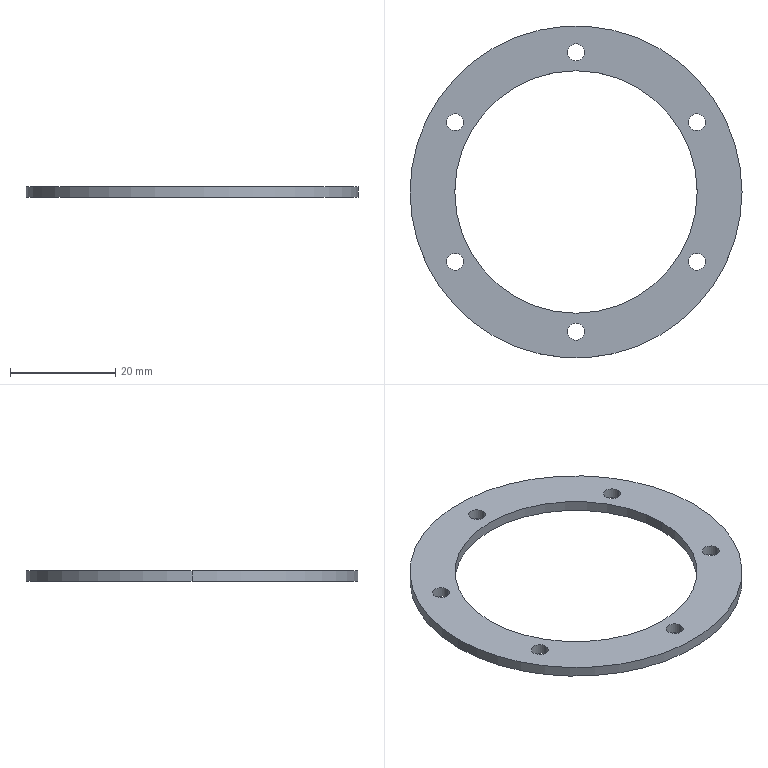Part | SolidWorks | features BaseBody 1 | 1 solid | 18 faces | box 63 x 63 x 2 mm | volume 2814 mm3 | cylinder 16 | plane 2 | commonest cylinder face diameters 3.2 x12 46 x2 63 x2
STEP:
#1=CARTESIAN_POINT('',(-21.35,13.25,2.));
#2=VERTEX_POINT('',#1);
#3=CARTESIAN_POINT('',(-24.55,13.25,2.));
#4=VERTEX_POINT('',#3);
#5=CARTESIAN_POINT('',(-22.95,13.25,2.));
#6=DIRECTION('',(0.,0.,-1.));
#7=DIRECTION('',(-1.,0.,0.));
#8=AXIS2_PLACEMENT_3D('',#5,#6,#7);
#9=CIRCLE('',#8,1.6);
#10=EDGE_CURVE('',#2,#4,#9,.T.);
#11=ORIENTED_EDGE('',*,*,#10,.F.);
#12=CARTESIAN_POINT('',(-21.35,13.25,0.));
#13=VERTEX_POINT('',#12);
#14=CARTESIAN_POINT('',(-21.35,13.25,2.));
#15=DIRECTION('',(0.,0.,-1.));
#16=VECTOR('',#15,1000.);
#17=LINE('',#14,#16);
#18=EDGE_CURVE('',#2,#13,#17,.T.);
#19=ORIENTED_EDGE('',*,*,#18,.T.);
#20=CARTESIAN_POINT('',(-24.55,13.25,0.));
#21=VERTEX_POINT('',#20);
#22=CARTESIAN_POINT('',(-22.95,13.25,0.));
#23=DIRECTION('',(0.,0.,1.));
#24=DIRECTION('',(-1.,0.,0.));
#25=AXIS2_PLACEMENT_3D('',#22,#23,#24);
#26=CIRCLE('',#25,1.6);
#27=EDGE_CURVE('',#21,#13,#26,.T.);
#28=ORIENTED_EDGE('',*,*,#27,.F.);
#29=CARTESIAN_POINT('',(-24.55,13.25,2.));
#30=DIRECTION('',(0.,0.,-1.));
#31=VECTOR('',#30,1000.);
#32=LINE('',#29,#31);
#33=EDGE_CURVE('',#4,#21,#32,.T.);
#34=ORIENTED_EDGE('',*,*,#33,.F.);
#35=EDGE_LOOP('',(#11,#19,#28,#34));
#36=FACE_OUTER_BOUND('',#35,.T.);
#37=CARTESIAN_POINT('',(-22.95,13.25,2.));
#38=DIRECTION('',(0.,0.,-1.));
#39=DIRECTION('',(-1.,0.,0.));
#40=AXIS2_PLACEMENT_3D('',#37,#38,#39);
#41=CYLINDRICAL_SURFACE('',#40,1.6);
#42=ADVANCED_FACE('',(#36),#41,.F.);
#43=CARTESIAN_POINT('',(1.6,-26.5,2.));
#44=VERTEX_POINT('',#43);
#45=CARTESIAN_POINT('',(-1.6,-26.5,2.));
#46=VERTEX_POINT('',#45);
#47=CARTESIAN_POINT('',(0.,-26.5,2.));
#48=DIRECTION('',(0.,0.,-1.));
#49=DIRECTION('',(-1.,0.,0.));
#50=AXIS2_PLACEMENT_3D('',#47,#48,#49);
#51=CIRCLE('',#50,1.6);
#52=EDGE_CURVE('',#44,#46,#51,.T.);
#53=ORIENTED_EDGE('',*,*,#52,.F.);
#54=CARTESIAN_POINT('',(1.6,-26.5,0.));
#55=VERTEX_POINT('',#54);
#56=CARTESIAN_POINT('',(1.6,-26.5,2.));
#57=DIRECTION('',(0.,0.,-1.));
#58=VECTOR('',#57,1000.);
#59=LINE('',#56,#58);
#60=EDGE_CURVE('',#44,#55,#59,.T.);
#61=ORIENTED_EDGE('',*,*,#60,.T.);
#62=CARTESIAN_POINT('',(-1.6,-26.5,0.));
#63=VERTEX_POINT('',#62);
#64=CARTESIAN_POINT('',(0.,-26.5,0.));
#65=DIRECTION('',(0.,0.,1.));
#66=DIRECTION('',(-1.,0.,0.));
#67=AXIS2_PLACEMENT_3D('',#64,#65,#66);
#68=CIRCLE('',#67,1.6);
#69=EDGE_CURVE('',#63,#55,#68,.T.);
#70=ORIENTED_EDGE('',*,*,#69,.F.);
#71=CARTESIAN_POINT('',(-1.6,-26.5,2.));
#72=DIRECTION('',(0.,0.,-1.));
#73=VECTOR('',#72,1000.);
#74=LINE('',#71,#73);
#75=EDGE_CURVE('',#46,#63,#74,.T.);
#76=ORIENTED_EDGE('',*,*,#75,.F.);
#77=EDGE_LOOP('',(#53,#61,#70,#76));
#78=FACE_OUTER_BOUND('',#77,.T.);
#79=CARTESIAN_POINT('',(0.,-26.5,2.));
#80=DIRECTION('',(0.,0.,-1.));
#81=DIRECTION('',(-1.,0.,0.));
#82=AXIS2_PLACEMENT_3D('',#79,#80,#81);
#83=CYLINDRICAL_SURFACE('',#82,1.6);
#84=ADVANCED_FACE('',(#78),#83,.F.);
#85=CARTESIAN_POINT('',(24.55,13.25,2.));
#86=VERTEX_POINT('',#85);
#87=CARTESIAN_POINT('',(21.35,13.25,2.));
#88=VERTEX_POINT('',#87);
#89=CARTESIAN_POINT('',(22.95,13.25,2.));
#90=DIRECTION('',(0.,0.,-1.));
#91=DIRECTION('',(-1.,0.,0.));
#92=AXIS2_PLACEMENT_3D('',#89,#90,#91);
#93=CIRCLE('',#92,1.6);
#94=EDGE_CURVE('',#86,#88,#93,.T.);
#95=ORIENTED_EDGE('',*,*,#94,.F.);
#96=CARTESIAN_POINT('',(24.55,13.25,0.));
#97=VERTEX_POINT('',#96);
#98=CARTESIAN_POINT('',(24.55,13.25,2.));
#99=DIRECTION('',(0.,0.,-1.));
#100=VECTOR('',#99,1000.);
#101=LINE('',#98,#100);
#102=EDGE_CURVE('',#86,#97,#101,.T.);
#103=ORIENTED_EDGE('',*,*,#102,.T.);
#104=CARTESIAN_POINT('',(21.35,13.25,0.));
#105=VERTEX_POINT('',#104);
#106=CARTESIAN_POINT('',(22.95,13.25,0.));
#107=DIRECTION('',(0.,0.,1.));
#108=DIRECTION('',(-1.,0.,0.));
#109=AXIS2_PLACEMENT_3D('',#106,#107,#108);
#110=CIRCLE('',#109,1.6);
#111=EDGE_CURVE('',#105,#97,#110,.T.);
#112=ORIENTED_EDGE('',*,*,#111,.F.);
#113=CARTESIAN_POINT('',(21.35,13.25,2.));
#114=DIRECTION('',(0.,0.,-1.));
#115=VECTOR('',#114,1000.);
#116=LINE('',#113,#115);
#117=EDGE_CURVE('',#88,#105,#116,.T.);
#118=ORIENTED_EDGE('',*,*,#117,.F.);
#119=EDGE_LOOP('',(#95,#103,#112,#118));
#120=FACE_OUTER_BOUND('',#119,.T.);
#121=CARTESIAN_POINT('',(22.95,13.25,2.));
#122=DIRECTION('',(0.,0.,-1.));
#123=DIRECTION('',(-1.,0.,0.));
#124=AXIS2_PLACEMENT_3D('',#121,#122,#123);
#125=CYLINDRICAL_SURFACE('',#124,1.6);
#126=ADVANCED_FACE('',(#120),#125,.F.);
#127=CARTESIAN_POINT('',(23.,0.,2.));
#128=VERTEX_POINT('',#127);
#129=CARTESIAN_POINT('',(-23.,0.,2.));
#130=VERTEX_POINT('',#129);
#131=CARTESIAN_POINT('',(0.,0.,2.));
#132=DIRECTION('',(0.,0.,-1.));
#133=DIRECTION('',(-1.,0.,0.));
#134=AXIS2_PLACEMENT_3D('',#131,#132,#133);
#135=CIRCLE('',#134,23.);
#136=EDGE_CURVE('',#128,#130,#135,.T.);
#137=ORIENTED_EDGE('',*,*,#136,.F.);
#138=CARTESIAN_POINT('',(23.,0.,0.));
#139=VERTEX_POINT('',#138);
#140=CARTESIAN_POINT('',(23.,0.,2.));
#141=DIRECTION('',(0.,0.,-1.));
#142=VECTOR('',#141,1000.);
#143=LINE('',#140,#142);
#144=EDGE_CURVE('',#128,#139,#143,.T.);
#145=ORIENTED_EDGE('',*,*,#144,.T.);
#146=CARTESIAN_POINT('',(-23.,0.,0.));
#147=VERTEX_POINT('',#146);
#148=CARTESIAN_POINT('',(0.,0.,0.));
#149=DIRECTION('',(0.,0.,1.));
#150=DIRECTION('',(-1.,0.,0.));
#151=AXIS2_PLACEMENT_3D('',#148,#149,#150);
#152=CIRCLE('',#151,23.);
#153=EDGE_CURVE('',#147,#139,#152,.T.);
#154=ORIENTED_EDGE('',*,*,#153,.F.);
#155=CARTESIAN_POINT('',(-23.,0.,2.));
#156=DIRECTION('',(0.,0.,-1.));
#157=VECTOR('',#156,1000.);
#158=LINE('',#155,#157);
#159=EDGE_CURVE('',#130,#147,#158,.T.);
#160=ORIENTED_EDGE('',*,*,#159,.F.);
#161=EDGE_LOOP('',(#137,#145,#154,#160));
#162=FACE_OUTER_BOUND('',#161,.T.);
#163=CARTESIAN_POINT('',(0.,0.,2.));
#164=DIRECTION('',(0.,0.,-1.));
#165=DIRECTION('',(-1.,0.,0.));
#166=AXIS2_PLACEMENT_3D('',#163,#164,#165);
#167=CYLINDRICAL_SURFACE('',#166,23.);
#168=ADVANCED_FACE('',(#162),#167,.F.);
#169=CARTESIAN_POINT('',(31.5,0.,2.));
#170=VERTEX_POINT('',#169);
#171=CARTESIAN_POINT('',(-31.5,0.,2.));
#172=VERTEX_POINT('',#171);
#173=CARTESIAN_POINT('',(0.,0.,2.));
#174=DIRECTION('',(0.,0.,1.));
#175=DIRECTION('',(-1.,0.,0.));
#176=AXIS2_PLACEMENT_3D('',#173,#174,#175);
#177=CIRCLE('',#176,31.5);
#178=EDGE_CURVE('',#170,#172,#177,.T.);
#179=ORIENTED_EDGE('',*,*,#178,.F.);
#180=CARTESIAN_POINT('',(31.5,0.,0.));
#181=VERTEX_POINT('',#180);
#182=CARTESIAN_POINT('',(31.5,0.,2.));
#183=DIRECTION('',(0.,0.,-1.));
#184=VECTOR('',#183,1000.);
#185=LINE('',#182,#184);
#186=EDGE_CURVE('',#170,#181,#185,.T.);
#187=ORIENTED_EDGE('',*,*,#186,.T.);
#188=CARTESIAN_POINT('',(-31.5,0.,0.));
#189=VERTEX_POINT('',#188);
#190=CARTESIAN_POINT('',(0.,0.,0.));
#191=DIRECTION('',(0.,0.,1.));
#192=DIRECTION('',(-1.,0.,0.));
#193=AXIS2_PLACEMENT_3D('',#190,#191,#192);
#194=CIRCLE('',#193,31.5);
#195=EDGE_CURVE('',#181,#189,#194,.T.);
#196=ORIENTED_EDGE('',*,*,#195,.T.);
#197=CARTESIAN_POINT('',(-31.5,0.,2.));
#198=DIRECTION('',(0.,0.,-1.));
#199=VECTOR('',#198,1000.);
#200=LINE('',#197,#199);
#201=EDGE_CURVE('',#172,#189,#200,.T.);
#202=ORIENTED_EDGE('',*,*,#201,.F.);
#203=EDGE_LOOP('',(#179,#187,#196,#202));
#204=FACE_OUTER_BOUND('',#203,.T.);
#205=CARTESIAN_POINT('',(0.,0.,2.));
#206=DIRECTION('',(0.,0.,-1.));
#207=DIRECTION('',(-1.,0.,0.));
#208=AXIS2_PLACEMENT_3D('',#205,#206,#207);
#209=CYLINDRICAL_SURFACE('',#208,31.5);
#210=ADVANCED_FACE('',(#204),#209,.T.);
#211=CARTESIAN_POINT('',(1.6,26.5,2.));
#212=VERTEX_POINT('',#211);
#213=CARTESIAN_POINT('',(-1.6,26.5,2.));
#214=VERTEX_POINT('',#213);
#215=CARTESIAN_POINT('',(0.,26.5,2.));
#216=DIRECTION('',(0.,0.,-1.));
#217=DIRECTION('',(-1.,0.,0.));
#218=AXIS2_PLACEMENT_3D('',#215,#216,#217);
#219=CIRCLE('',#218,1.6);
#220=EDGE_CURVE('',#212,#214,#219,.T.);
#221=ORIENTED_EDGE('',*,*,#220,.F.);
#222=CARTESIAN_POINT('',(1.6,26.5,0.));
#223=VERTEX_POINT('',#222);
#224=CARTESIAN_POINT('',(1.6,26.5,2.));
#225=DIRECTION('',(0.,0.,-1.));
#226=VECTOR('',#225,1000.);
#227=LINE('',#224,#226);
#228=EDGE_CURVE('',#212,#223,#227,.T.);
#229=ORIENTED_EDGE('',*,*,#228,.T.);
#230=CARTESIAN_POINT('',(-1.6,26.5,0.));
#231=VERTEX_POINT('',#230);
#232=CARTESIAN_POINT('',(0.,26.5,0.));
#233=DIRECTION('',(0.,0.,1.));
#234=DIRECTION('',(-1.,0.,0.));
#235=AXIS2_PLACEMENT_3D('',#232,#233,#234);
#236=CIRCLE('',#235,1.6);
#237=EDGE_CURVE('',#231,#223,#236,.T.);
#238=ORIENTED_EDGE('',*,*,#237,.F.);
#239=CARTESIAN_POINT('',(-1.6,26.5,2.));
#240=DIRECTION('',(0.,0.,-1.));
#241=VECTOR('',#240,1000.);
#242=LINE('',#239,#241);
#243=EDGE_CURVE('',#214,#231,#242,.T.);
#244=ORIENTED_EDGE('',*,*,#243,.F.);
#245=EDGE_LOOP('',(#221,#229,#238,#244));
#246=FACE_OUTER_BOUND('',#245,.T.);
#247=CARTESIAN_POINT('',(0.,26.5,2.));
#248=DIRECTION('',(0.,0.,-1.));
#249=DIRECTION('',(-1.,0.,0.));
#250=AXIS2_PLACEMENT_3D('',#247,#248,#249);
#251=CYLINDRICAL_SURFACE('',#250,1.6);
#252=ADVANCED_FACE('',(#246),#251,.F.);
#253=CARTESIAN_POINT('',(24.55,-13.25,2.));
#254=VERTEX_POINT('',#253);
#255=CARTESIAN_POINT('',(21.35,-13.25,2.));
#256=VERTEX_POINT('',#255);
#257=CARTESIAN_POINT('',(22.95,-13.25,2.));
#258=DIRECTION('',(0.,0.,-1.));
#259=DIRECTION('',(-1.,0.,0.));
#260=AXIS2_PLACEMENT_3D('',#257,#258,#259);
#261=CIRCLE('',#260,1.6);
#262=EDGE_CURVE('',#254,#256,#261,.T.);
#263=ORIENTED_EDGE('',*,*,#262,.F.);
#264=CARTESIAN_POINT('',(24.55,-13.25,0.));
#265=VERTEX_POINT('',#264);
#266=CARTESIAN_POINT('',(24.55,-13.25,2.));
#267=DIRECTION('',(0.,0.,-1.));
#268=VECTOR('',#267,1000.);
#269=LINE('',#266,#268);
#270=EDGE_CURVE('',#254,#265,#269,.T.);
#271=ORIENTED_EDGE('',*,*,#270,.T.);
#272=CARTESIAN_POINT('',(21.35,-13.25,0.));
#273=VERTEX_POINT('',#272);
#274=CARTESIAN_POINT('',(22.95,-13.25,0.));
#275=DIRECTION('',(0.,0.,1.));
#276=DIRECTION('',(-1.,0.,0.));
#277=AXIS2_PLACEMENT_3D('',#274,#275,#276);
#278=CIRCLE('',#277,1.6);
#279=EDGE_CURVE('',#273,#265,#278,.T.);
#280=ORIENTED_EDGE('',*,*,#279,.F.);
#281=CARTESIAN_POINT('',(21.35,-13.25,2.));
#282=DIRECTION('',(0.,0.,-1.));
#283=VECTOR('',#282,1000.);
#284=LINE('',#281,#283);
#285=EDGE_CURVE('',#256,#273,#284,.T.);
#286=ORIENTED_EDGE('',*,*,#285,.F.);
#287=EDGE_LOOP('',(#263,#271,#280,#286));
#288=FACE_OUTER_BOUND('',#287,.T.);
#289=CARTESIAN_POINT('',(22.95,-13.25,2.));
#290=DIRECTION('',(0.,0.,-1.));
#291=DIRECTION('',(-1.,0.,0.));
#292=AXIS2_PLACEMENT_3D('',#289,#290,#291);
#293=CYLINDRICAL_SURFACE('',#292,1.6);
#294=ADVANCED_FACE('',(#288),#293,.F.);
#295=CARTESIAN_POINT('',(-21.35,-13.25,2.));
#296=VERTEX_POINT('',#295);
#297=CARTESIAN_POINT('',(-24.55,-13.25,2.));
#298=VERTEX_POINT('',#297);
#299=CARTESIAN_POINT('',(-22.95,-13.25,2.));
#300=DIRECTION('',(0.,0.,-1.));
#301=DIRECTION('',(-1.,0.,0.));
#302=AXIS2_PLACEMENT_3D('',#299,#300,#301);
#303=CIRCLE('',#302,1.6);
#304=EDGE_CURVE('',#296,#298,#303,.T.);
#305=ORIENTED_EDGE('',*,*,#304,.F.);
#306=CARTESIAN_POINT('',(-21.35,-13.25,0.));
#307=VERTEX_POINT('',#306);
#308=CARTESIAN_POINT('',(-21.35,-13.25,2.));
#309=DIRECTION('',(0.,0.,-1.));
#310=VECTOR('',#309,1000.);
#311=LINE('',#308,#310);
#312=EDGE_CURVE('',#296,#307,#311,.T.);
#313=ORIENTED_EDGE('',*,*,#312,.T.);
#314=CARTESIAN_POINT('',(-24.55,-13.25,0.));
#315=VERTEX_POINT('',#314);
#316=CARTESIAN_POINT('',(-22.95,-13.25,0.));
#317=DIRECTION('',(0.,0.,1.));
#318=DIRECTION('',(-1.,0.,0.));
#319=AXIS2_PLACEMENT_3D('',#316,#317,#318);
#320=CIRCLE('',#319,1.6);
#321=EDGE_CURVE('',#315,#307,#320,.T.);
#322=ORIENTED_EDGE('',*,*,#321,.F.);
#323=CARTESIAN_POINT('',(-24.55,-13.25,2.));
#324=DIRECTION('',(0.,0.,-1.));
#325=VECTOR('',#324,1000.);
#326=LINE('',#323,#325);
#327=EDGE_CURVE('',#298,#315,#326,.T.);
#328=ORIENTED_EDGE('',*,*,#327,.F.);
#329=EDGE_LOOP('',(#305,#313,#322,#328));
#330=FACE_OUTER_BOUND('',#329,.T.);
#331=CARTESIAN_POINT('',(-22.95,-13.25,2.));
#332=DIRECTION('',(0.,0.,-1.));
#333=DIRECTION('',(-1.,0.,0.));
#334=AXIS2_PLACEMENT_3D('',#331,#332,#333);
#335=CYLINDRICAL_SURFACE('',#334,1.6);
#336=ADVANCED_FACE('',(#330),#335,.F.);
#337=CARTESIAN_POINT('',(-22.95,13.25,2.));
#338=DIRECTION('',(0.,0.,-1.));
#339=DIRECTION('',(-1.,0.,0.));
#340=AXIS2_PLACEMENT_3D('',#337,#338,#339);
#341=CIRCLE('',#340,1.6);
#342=EDGE_CURVE('',#4,#2,#341,.T.);
#343=ORIENTED_EDGE('',*,*,#342,.T.);
#344=ORIENTED_EDGE('',*,*,#10,.T.);
#345=EDGE_LOOP('',(#343,#344));
#346=FACE_BOUND('',#345,.T.);
#347=CARTESIAN_POINT('',(0.,-26.5,2.));
#348=DIRECTION('',(0.,0.,-1.));
#349=DIRECTION('',(-1.,0.,0.));
#350=AXIS2_PLACEMENT_3D('',#347,#348,#349);
#351=CIRCLE('',#350,1.6);
#352=EDGE_CURVE('',#46,#44,#351,.T.);
#353=ORIENTED_EDGE('',*,*,#352,.T.);
#354=ORIENTED_EDGE('',*,*,#52,.T.);
#355=EDGE_LOOP('',(#353,#354));
#356=FACE_BOUND('',#355,.T.);
#357=CARTESIAN_POINT('',(22.95,13.25,2.));
#358=DIRECTION('',(0.,0.,-1.));
#359=DIRECTION('',(-1.,0.,0.));
#360=AXIS2_PLACEMENT_3D('',#357,#358,#359);
#361=CIRCLE('',#360,1.6);
#362=EDGE_CURVE('',#88,#86,#361,.T.);
#363=ORIENTED_EDGE('',*,*,#362,.T.);
#364=ORIENTED_EDGE('',*,*,#94,.T.);
#365=EDGE_LOOP('',(#363,#364));
#366=FACE_BOUND('',#365,.T.);
#367=CARTESIAN_POINT('',(0.,0.,2.));
#368=DIRECTION('',(0.,0.,-1.));
#369=DIRECTION('',(-1.,0.,0.));
#370=AXIS2_PLACEMENT_3D('',#367,#368,#369);
#371=CIRCLE('',#370,23.);
#372=EDGE_CURVE('',#130,#128,#371,.T.);
#373=ORIENTED_EDGE('',*,*,#372,.T.);
#374=ORIENTED_EDGE('',*,*,#136,.T.);
#375=EDGE_LOOP('',(#373,#374));
#376=FACE_BOUND('',#375,.T.);
#377=CARTESIAN_POINT('',(0.,0.,2.));
#378=DIRECTION('',(0.,0.,1.));
#379=DIRECTION('',(-1.,0.,0.));
#380=AXIS2_PLACEMENT_3D('',#377,#378,#379);
#381=CIRCLE('',#380,31.5);
#382=EDGE_CURVE('',#172,#170,#381,.T.);
#383=ORIENTED_EDGE('',*,*,#382,.T.);
#384=ORIENTED_EDGE('',*,*,#178,.T.);
#385=EDGE_LOOP('',(#383,#384));
#386=FACE_OUTER_BOUND('',#385,.T.);
#387=CARTESIAN_POINT('',(0.,26.5,2.));
#388=DIRECTION('',(0.,0.,-1.));
#389=DIRECTION('',(-1.,0.,0.));
#390=AXIS2_PLACEMENT_3D('',#387,#388,#389);
#391=CIRCLE('',#390,1.6);
#392=EDGE_CURVE('',#214,#212,#391,.T.);
#393=ORIENTED_EDGE('',*,*,#392,.T.);
#394=ORIENTED_EDGE('',*,*,#220,.T.);
#395=EDGE_LOOP('',(#393,#394));
#396=FACE_BOUND('',#395,.T.);
#397=CARTESIAN_POINT('',(22.95,-13.25,2.));
#398=DIRECTION('',(0.,0.,-1.));
#399=DIRECTION('',(-1.,0.,0.));
#400=AXIS2_PLACEMENT_3D('',#397,#398,#399);
#401=CIRCLE('',#400,1.6);
#402=EDGE_CURVE('',#256,#254,#401,.T.);
#403=ORIENTED_EDGE('',*,*,#402,.T.);
#404=ORIENTED_EDGE('',*,*,#262,.T.);
#405=EDGE_LOOP('',(#403,#404));
#406=FACE_BOUND('',#405,.T.);
#407=CARTESIAN_POINT('',(-22.95,-13.25,2.));
#408=DIRECTION('',(0.,0.,-1.));
#409=DIRECTION('',(-1.,0.,0.));
#410=AXIS2_PLACEMENT_3D('',#407,#408,#409);
#411=CIRCLE('',#410,1.6);
#412=EDGE_CURVE('',#298,#296,#411,.T.);
#413=ORIENTED_EDGE('',*,*,#412,.T.);
#414=ORIENTED_EDGE('',*,*,#304,.T.);
#415=EDGE_LOOP('',(#413,#414));
#416=FACE_BOUND('',#415,.T.);
#417=CARTESIAN_POINT('',(0.,0.,2.));
#418=DIRECTION('',(0.,0.,1.));
#419=DIRECTION('',(1.,0.,0.));
#420=AXIS2_PLACEMENT_3D('',#417,#418,#419);
#421=PLANE('',#420);
#422=ADVANCED_FACE('',(#346,#356,#366,#376,#386,#396,#406,#416),#421,.T.);
#423=ORIENTED_EDGE('',*,*,#18,.F.);
#424=ORIENTED_EDGE('',*,*,#342,.F.);
#425=ORIENTED_EDGE('',*,*,#33,.T.);
#426=CARTESIAN_POINT('',(-22.95,13.25,0.));
#427=DIRECTION('',(0.,0.,1.));
#428=DIRECTION('',(-1.,0.,0.));
#429=AXIS2_PLACEMENT_3D('',#426,#427,#428);
#430=CIRCLE('',#429,1.6);
#431=EDGE_CURVE('',#13,#21,#430,.T.);
#432=ORIENTED_EDGE('',*,*,#431,.F.);
#433=EDGE_LOOP('',(#423,#424,#425,#432));
#434=FACE_OUTER_BOUND('',#433,.T.);
#435=CARTESIAN_POINT('',(-22.95,13.25,2.));
#436=DIRECTION('',(0.,0.,-1.));
#437=DIRECTION('',(-1.,0.,0.));
#438=AXIS2_PLACEMENT_3D('',#435,#436,#437);
#439=CYLINDRICAL_SURFACE('',#438,1.6);
#440=ADVANCED_FACE('',(#434),#439,.F.);
#441=ORIENTED_EDGE('',*,*,#60,.F.);
#442=ORIENTED_EDGE('',*,*,#352,.F.);
#443=ORIENTED_EDGE('',*,*,#75,.T.);
#444=CARTESIAN_POINT('',(0.,-26.5,0.));
#445=DIRECTION('',(0.,0.,1.));
#446=DIRECTION('',(-1.,0.,0.));
#447=AXIS2_PLACEMENT_3D('',#444,#445,#446);
#448=CIRCLE('',#447,1.6);
#449=EDGE_CURVE('',#55,#63,#448,.T.);
#450=ORIENTED_EDGE('',*,*,#449,.F.);
#451=EDGE_LOOP('',(#441,#442,#443,#450));
#452=FACE_OUTER_BOUND('',#451,.T.);
#453=CARTESIAN_POINT('',(0.,-26.5,2.));
#454=DIRECTION('',(0.,0.,-1.));
#455=DIRECTION('',(-1.,0.,0.));
#456=AXIS2_PLACEMENT_3D('',#453,#454,#455);
#457=CYLINDRICAL_SURFACE('',#456,1.6);
#458=ADVANCED_FACE('',(#452),#457,.F.);
#459=ORIENTED_EDGE('',*,*,#102,.F.);
#460=ORIENTED_EDGE('',*,*,#362,.F.);
#461=ORIENTED_EDGE('',*,*,#117,.T.);
#462=CARTESIAN_POINT('',(22.95,13.25,0.));
#463=DIRECTION('',(0.,0.,1.));
#464=DIRECTION('',(-1.,0.,0.));
#465=AXIS2_PLACEMENT_3D('',#462,#463,#464);
#466=CIRCLE('',#465,1.6);
#467=EDGE_CURVE('',#97,#105,#466,.T.);
#468=ORIENTED_EDGE('',*,*,#467,.F.);
#469=EDGE_LOOP('',(#459,#460,#461,#468));
#470=FACE_OUTER_BOUND('',#469,.T.);
#471=CARTESIAN_POINT('',(22.95,13.25,2.));
#472=DIRECTION('',(0.,0.,-1.));
#473=DIRECTION('',(-1.,0.,0.));
#474=AXIS2_PLACEMENT_3D('',#471,#472,#473);
#475=CYLINDRICAL_SURFACE('',#474,1.6);
#476=ADVANCED_FACE('',(#470),#475,.F.);
#477=ORIENTED_EDGE('',*,*,#144,.F.);
#478=ORIENTED_EDGE('',*,*,#372,.F.);
#479=ORIENTED_EDGE('',*,*,#159,.T.);
#480=CARTESIAN_POINT('',(0.,0.,0.));
#481=DIRECTION('',(0.,0.,1.));
#482=DIRECTION('',(-1.,0.,0.));
#483=AXIS2_PLACEMENT_3D('',#480,#481,#482);
#484=CIRCLE('',#483,23.);
#485=EDGE_CURVE('',#139,#147,#484,.T.);
#486=ORIENTED_EDGE('',*,*,#485,.F.);
#487=EDGE_LOOP('',(#477,#478,#479,#486));
#488=FACE_OUTER_BOUND('',#487,.T.);
#489=CARTESIAN_POINT('',(0.,0.,2.));
#490=DIRECTION('',(0.,0.,-1.));
#491=DIRECTION('',(-1.,0.,0.));
#492=AXIS2_PLACEMENT_3D('',#489,#490,#491);
#493=CYLINDRICAL_SURFACE('',#492,23.);
#494=ADVANCED_FACE('',(#488),#493,.F.);
#495=ORIENTED_EDGE('',*,*,#186,.F.);
#496=ORIENTED_EDGE('',*,*,#382,.F.);
#497=ORIENTED_EDGE('',*,*,#201,.T.);
#498=CARTESIAN_POINT('',(0.,0.,0.));
#499=DIRECTION('',(0.,0.,1.));
#500=DIRECTION('',(-1.,0.,0.));
#501=AXIS2_PLACEMENT_3D('',#498,#499,#500);
#502=CIRCLE('',#501,31.5);
#503=EDGE_CURVE('',#189,#181,#502,.T.);
#504=ORIENTED_EDGE('',*,*,#503,.T.);
#505=EDGE_LOOP('',(#495,#496,#497,#504));
#506=FACE_OUTER_BOUND('',#505,.T.);
#507=CARTESIAN_POINT('',(0.,0.,2.));
#508=DIRECTION('',(0.,0.,-1.));
#509=DIRECTION('',(-1.,0.,0.));
#510=AXIS2_PLACEMENT_3D('',#507,#508,#509);
#511=CYLINDRICAL_SURFACE('',#510,31.5);
#512=ADVANCED_FACE('',(#506),#511,.T.);
#513=ORIENTED_EDGE('',*,*,#228,.F.);
#514=ORIENTED_EDGE('',*,*,#392,.F.);
#515=ORIENTED_EDGE('',*,*,#243,.T.);
#516=CARTESIAN_POINT('',(0.,26.5,0.));
#517=DIRECTION('',(0.,0.,1.));
#518=DIRECTION('',(-1.,0.,0.));
#519=AXIS2_PLACEMENT_3D('',#516,#517,#518);
#520=CIRCLE('',#519,1.6);
#521=EDGE_CURVE('',#223,#231,#520,.T.);
#522=ORIENTED_EDGE('',*,*,#521,.F.);
#523=EDGE_LOOP('',(#513,#514,#515,#522));
#524=FACE_OUTER_BOUND('',#523,.T.);
#525=CARTESIAN_POINT('',(0.,26.5,2.));
#526=DIRECTION('',(0.,0.,-1.));
#527=DIRECTION('',(-1.,0.,0.));
#528=AXIS2_PLACEMENT_3D('',#525,#526,#527);
#529=CYLINDRICAL_SURFACE('',#528,1.6);
#530=ADVANCED_FACE('',(#524),#529,.F.);
#531=ORIENTED_EDGE('',*,*,#270,.F.);
#532=ORIENTED_EDGE('',*,*,#402,.F.);
#533=ORIENTED_EDGE('',*,*,#285,.T.);
#534=CARTESIAN_POINT('',(22.95,-13.25,0.));
#535=DIRECTION('',(0.,0.,1.));
#536=DIRECTION('',(-1.,0.,0.));
#537=AXIS2_PLACEMENT_3D('',#534,#535,#536);
#538=CIRCLE('',#537,1.6);
#539=EDGE_CURVE('',#265,#273,#538,.T.);
#540=ORIENTED_EDGE('',*,*,#539,.F.);
#541=EDGE_LOOP('',(#531,#532,#533,#540));
#542=FACE_OUTER_BOUND('',#541,.T.);
#543=CARTESIAN_POINT('',(22.95,-13.25,2.));
#544=DIRECTION('',(0.,0.,-1.));
#545=DIRECTION('',(-1.,0.,0.));
#546=AXIS2_PLACEMENT_3D('',#543,#544,#545);
#547=CYLINDRICAL_SURFACE('',#546,1.6);
#548=ADVANCED_FACE('',(#542),#547,.F.);
#549=ORIENTED_EDGE('',*,*,#312,.F.);
#550=ORIENTED_EDGE('',*,*,#412,.F.);
#551=ORIENTED_EDGE('',*,*,#327,.T.);
#552=CARTESIAN_POINT('',(-22.95,-13.25,0.));
#553=DIRECTION('',(0.,0.,1.));
#554=DIRECTION('',(-1.,0.,0.));
#555=AXIS2_PLACEMENT_3D('',#552,#553,#554);
#556=CIRCLE('',#555,1.6);
#557=EDGE_CURVE('',#307,#315,#556,.T.);
#558=ORIENTED_EDGE('',*,*,#557,.F.);
#559=EDGE_LOOP('',(#549,#550,#551,#558));
#560=FACE_OUTER_BOUND('',#559,.T.);
#561=CARTESIAN_POINT('',(-22.95,-13.25,2.));
#562=DIRECTION('',(0.,0.,-1.));
#563=DIRECTION('',(-1.,0.,0.));
#564=AXIS2_PLACEMENT_3D('',#561,#562,#563);
#565=CYLINDRICAL_SURFACE('',#564,1.6);
#566=ADVANCED_FACE('',(#560),#565,.F.);
#567=ORIENTED_EDGE('',*,*,#27,.T.);
#568=ORIENTED_EDGE('',*,*,#431,.T.);
#569=EDGE_LOOP('',(#567,#568));
#570=FACE_BOUND('',#569,.T.);
#571=ORIENTED_EDGE('',*,*,#321,.T.);
#572=ORIENTED_EDGE('',*,*,#557,.T.);
#573=EDGE_LOOP('',(#571,#572));
#574=FACE_BOUND('',#573,.T.);
#575=ORIENTED_EDGE('',*,*,#69,.T.);
#576=ORIENTED_EDGE('',*,*,#449,.T.);
#577=EDGE_LOOP('',(#575,#576));
#578=FACE_BOUND('',#577,.T.);
#579=ORIENTED_EDGE('',*,*,#279,.T.);
#580=ORIENTED_EDGE('',*,*,#539,.T.);
#581=EDGE_LOOP('',(#579,#580));
#582=FACE_BOUND('',#581,.T.);
#583=ORIENTED_EDGE('',*,*,#111,.T.);
#584=ORIENTED_EDGE('',*,*,#467,.T.);
#585=EDGE_LOOP('',(#583,#584));
#586=FACE_BOUND('',#585,.T.);
#587=ORIENTED_EDGE('',*,*,#237,.T.);
#588=ORIENTED_EDGE('',*,*,#521,.T.);
#589=EDGE_LOOP('',(#587,#588));
#590=FACE_BOUND('',#589,.T.);
#591=ORIENTED_EDGE('',*,*,#153,.T.);
#592=ORIENTED_EDGE('',*,*,#485,.T.);
#593=EDGE_LOOP('',(#591,#592));
#594=FACE_BOUND('',#593,.T.);
#595=ORIENTED_EDGE('',*,*,#503,.F.);
#596=ORIENTED_EDGE('',*,*,#195,.F.);
#597=EDGE_LOOP('',(#595,#596));
#598=FACE_OUTER_BOUND('',#597,.T.);
#599=CARTESIAN_POINT('',(0.,0.,0.));
#600=DIRECTION('',(0.,0.,1.));
#601=DIRECTION('',(1.,0.,0.));
#602=AXIS2_PLACEMENT_3D('',#599,#600,#601);
#603=PLANE('',#602);
#604=ADVANCED_FACE('',(#570,#574,#578,#582,#586,#590,#594,#598),#603,.F.);
#605=CLOSED_SHELL('',(#42,#84,#126,#168,#210,#252,#294,#336,#422,#440,#458,#476,#494,#512,#530,#548,#566,#604));
#606=MANIFOLD_SOLID_BREP('',#605);
#607=CARTESIAN_POINT('',(0.,0.,0.));
#608=DIRECTION('',(0.,0.,1.));
#609=DIRECTION('',(1.,0.,0.));
#610=AXIS2_PLACEMENT_3D('',#607,#608,#609);
#611=(LENGTH_UNIT()NAMED_UNIT(*)SI_UNIT(.MILLI.,.METRE.));
#612=UNCERTAINTY_MEASURE_WITH_UNIT(LENGTH_MEASURE(0.00001),#611,'','');
#613=(NAMED_UNIT(*)PLANE_ANGLE_UNIT()SI_UNIT($,.RADIAN.));
#614=(NAMED_UNIT(*)SI_UNIT($,.STERADIAN.)SOLID_ANGLE_UNIT());
#615=(GEOMETRIC_REPRESENTATION_CONTEXT(3)GLOBAL_UNCERTAINTY_ASSIGNED_CONTEXT((#612))GLOBAL_UNIT_ASSIGNED_CONTEXT((#611,#613,#614))REPRESENTATION_CONTEXT('',''));
#616=ADVANCED_BREP_SHAPE_REPRESENTATION('',(#606,#610),#615);